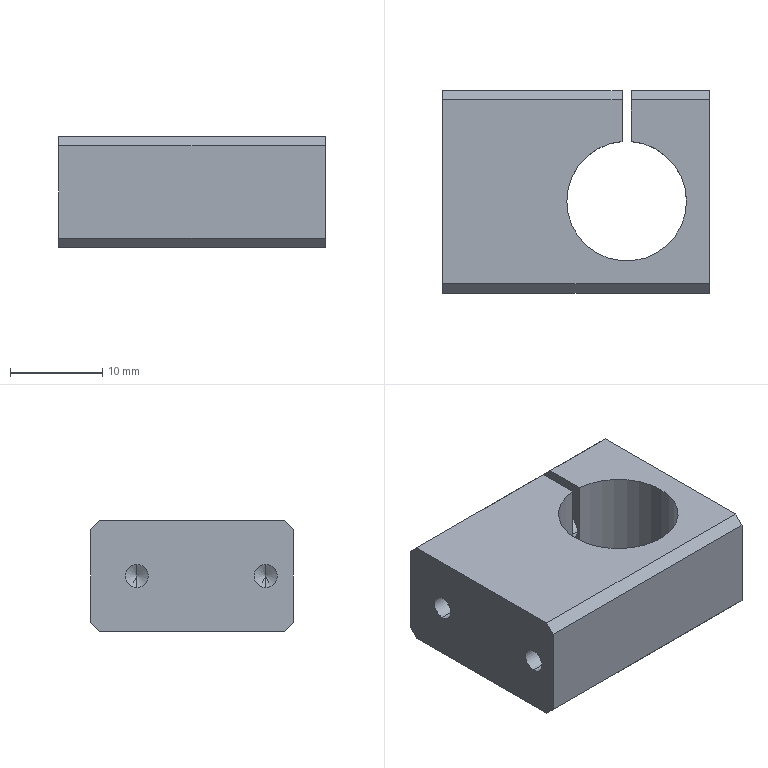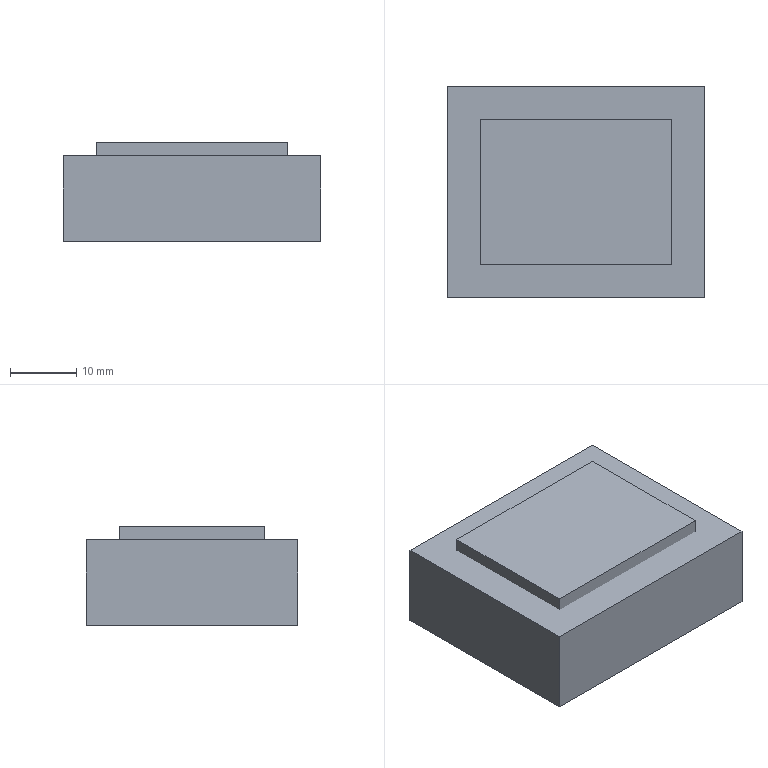CAM job | NX | 3+2 milling, drilling | part box 29 x 22 x 12 mm | stock box 39 x 32 x 15 mm
Tools:
number,name,description,diameter,corner_radius,flute_length,length,flutes
3,D63,Milling Tool-5 Parameters,63.0,0.0,50.0,75.0,2
1,D6A45,Milling Tool-5 Parameters,6.0,0.0,3.0,3.0,2
4,D10,Milling Tool-5 Parameters,10.0,0.0,50.0,75.0,2
16,D6JING,Milling Tool-5 Parameters,6.0,0.0,50.0,75.0,2
13,3.4ZT,Drilling Tool,3.4,0.0,35.0,50.0,2
12,2.5ZT,Drilling Tool,2.5,0.0,35.0,50.0,2
4,D4,Milling Tool-5 Parameters,4.0,0.0,50.0,75.0,2
11,2.3XYD,Thread Mill,2.3,0.0,0.5,50.0,2
20,D1,Milling Tool-5 Parameters,1.0,0.0,50.0,75.0,2
Operations:
program,operation,operation_type,tool,method,geometry_group,spindle_rpm,surface_speed,feed_per_tooth,feed_cut,feed_plunge,cut_length_mm,path_length_mm,cut_time_min,machine_time_min
1,FLOOR_WALL_COPY,VolumeBased25DMillingOperation,D63,METHOD,A,6500.0,1286.0,0.0962,1250.0,100.0,103.998,157.998,0.0832,0.0886
1,ADAPTIVE_MILLING_COPY,CavityMilling,D10,METHOD,A,9500.0,298.0,0.1842,3500.0,1000.0,848.012,928.012,0.243,0.251
1,HOLE_MILLING,CylinderMilling,D10,METHOD,A,9500.0,298.0,0.1053,2000.0,100.0,123.859,195.359,0.0619,0.0691
1,ZLEVEL_PROFILE_1_COPY,ZLevelMilling,D6JING,METHOD,A,9500.0,298.0,0.0526,1000.0,100.0,124.734,206.734,0.1247,0.1329
1,11_COPY_COPY,ZLevelMilling,D6A45,METHOD,A,9500.0,179.0,0.0526,1000.0,100.0,157.705,290.374,0.1577,0.171
1,CUTTERCOMP16,CylinderMilling,D6JING,METHOD,A,9500.0,179.0,0.0526,1000.0,100.0,123.765,195.265,0.1238,0.1309
2,FLOOR_WALL_COPY_COPY,VolumeBased25DMillingOperation,D63,METHOD,B,6500.0,1286.0,0.0962,1250.0,100.0,311.994,663.99,0.2496,0.2848
2,11_COPY_COPY_COPY,ZLevelMilling,D6A45,METHOD,B,9500.0,179.0,0.0526,1000.0,100.0,157.705,298.627,0.1577,0.1718
3,DRILLING_COPY_1,Operation,D6A45,METHOD,C,5000.0,94.0,0.025,250.0,0.0,4.0,68.0,0.016,0.0224
3,DRILLING_COPY_1_COPY_COPY,Operation,2.5ZT,METHOD,C,2000.0,21.0,0.0375,150.0,0.0,21.251,102.502,0.1417,0.1498
3,DRILLING_COPY_1_COPY,Operation,3.4ZT,METHOD,C,2000.0,21.0,0.0375,150.0,0.0,13.021,86.043,0.0868,0.0941
3,HOLE_MILLING_1,CylinderMilling,D4,METHOD,C,9500.0,119.0,0.0684,1300.0,100.0,91.199,154.099,0.0702,0.0764
3,11_COPY_COPY_COPY_COPY,ZLevelMilling,D6A45,METHOD,C,9500.0,179.0,0.0526,1000.0,100.0,102.81,235.526,0.1028,0.1161
3,CUTTERCOMP11,ThreadMilling,2.3XYD,METHOD,C,5000.0,36.0,0.085,850.0,100.0,102.353,358.853,0.1204,0.1461
4,DRILLING_COPY_1_COPY_1,Operation,D6A45,METHOD,D,5000.0,94.0,0.025,250.0,0.0,9.2,95.718,0.0368,0.0455
4,DRILLING_COPY_1_COPY_COPY_COPY,Operation,2.5ZT,METHOD,D,2000.0,21.0,0.0375,150.0,0.0,42.502,162.322,0.2833,0.2953
4,CUTTERCOMP11_COPY,ThreadMilling,2.3XYD,METHOD,D,5000.0,36.0,0.085,850.0,100.0,194.187,604.187,0.2285,0.2695
5,PLANAR_PROFILE,PlanarMilling,D1,METHOD,E,9500.0,29.0,0.0447,850.0,100.0,1387.0,1458.4,1.632,1.639